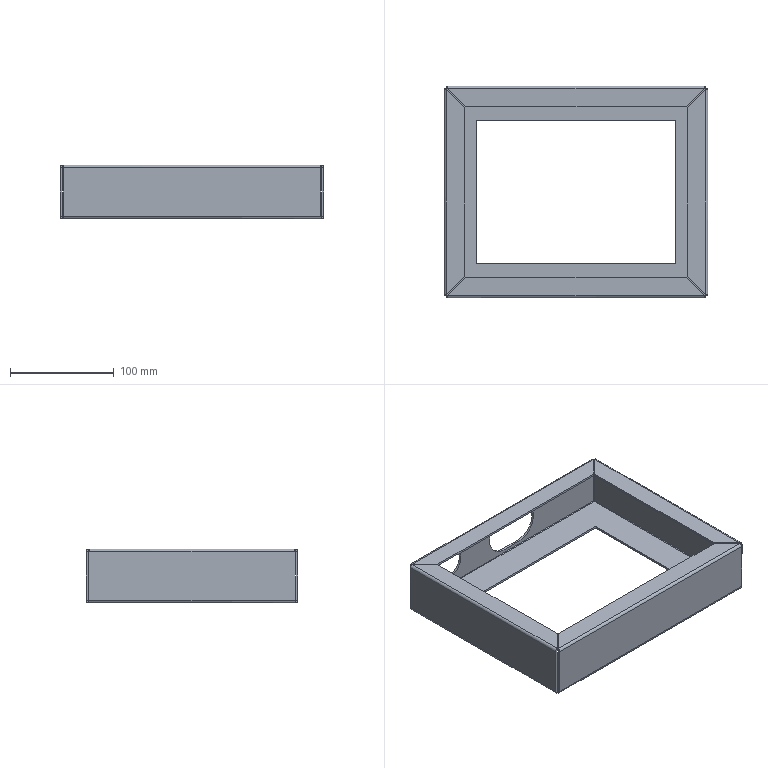Part | SolidWorks | features Cut 3, EdgeFlange 2, FlatPattern 1, ICE 1, SMBaseFlange 1, SheetMetal 1 | 1 solid | 80 faces | box 254 x 204 x 52 mm | volume 161787 mm3 | plane 44 | cylinder 20 | spline 16 | commonest cylinder face diameters 1 x8 5 x8 30 x2 40 x2